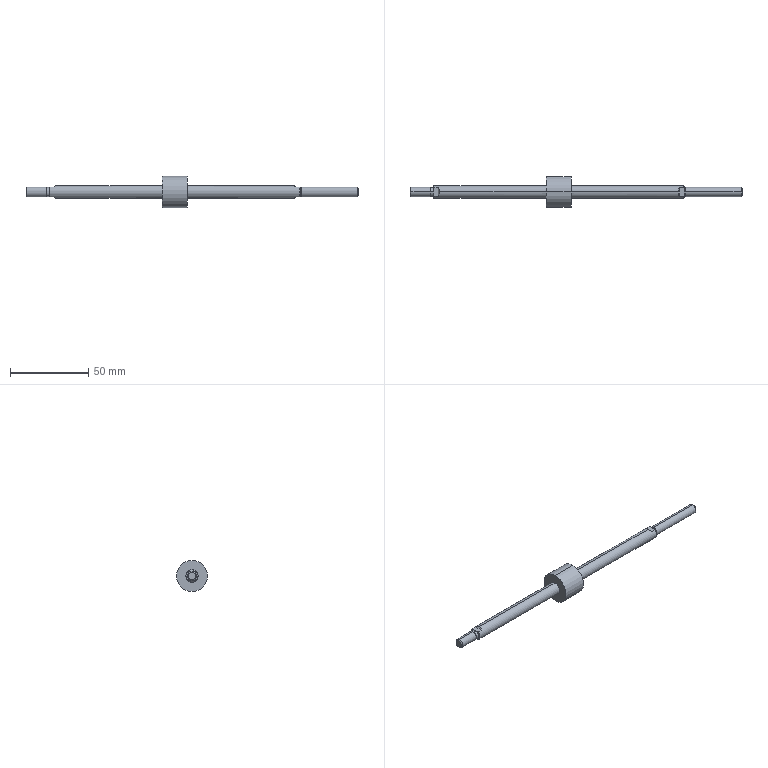Part | STEP file | 001-006-SDAJS_20x60_B2060_r | 1 solid | 38 faces | box 212.5 x 19.9 x 19.9 mm | volume 13647 mm3 | plane 16 | cylinder 14 | cone 8 | commonest cylinder face diameters 5.8 x4 6 x4 8 x4 19.9 x2